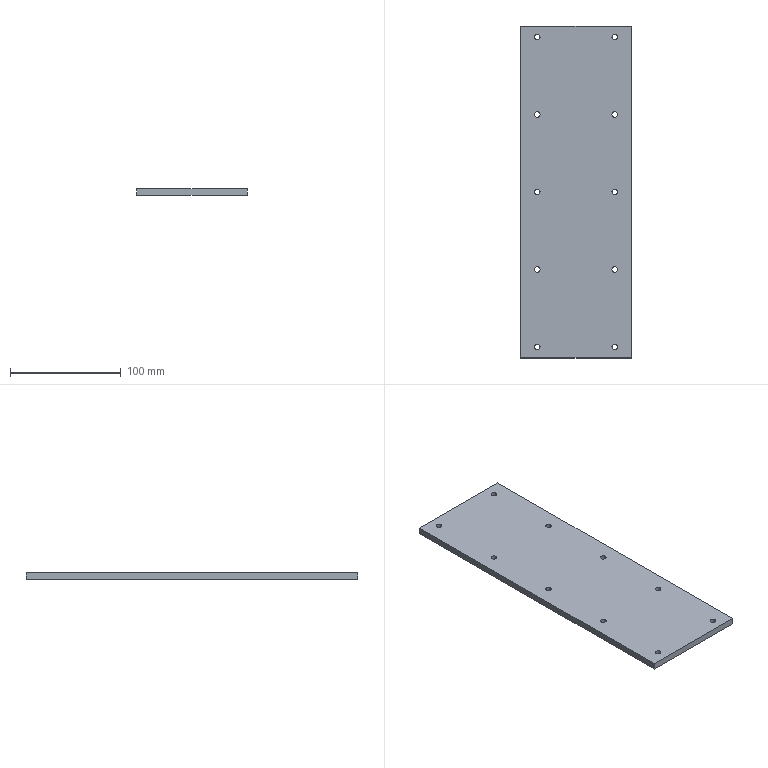Part | SolidWorks | features LPattern 2, Extrusion 1, HoleWzd 1 | 1 solid | 26 faces | box 100 x 300 x 6 mm | volume 178822 mm3 | cylinder 20 | plane 6 | commonest cylinder face diameters 5 x20
STEP:
#1=CARTESIAN_POINT('',(32.5,140.,0.));
#2=VERTEX_POINT('',#1);
#3=CARTESIAN_POINT('',(37.5,140.,0.));
#4=VERTEX_POINT('',#3);
#5=CARTESIAN_POINT('',(35.,140.,0.));
#6=DIRECTION('',(0.,0.,1.));
#7=DIRECTION('',(1.,0.,0.));
#8=AXIS2_PLACEMENT_3D('',#5,#6,#7);
#9=CIRCLE('',#8,2.5);
#10=EDGE_CURVE('',#2,#4,#9,.T.);
#11=ORIENTED_EDGE('',*,*,#10,.F.);
#12=CARTESIAN_POINT('',(32.5,140.,6.));
#13=VERTEX_POINT('',#12);
#14=CARTESIAN_POINT('',(32.5,140.,6.));
#15=DIRECTION('',(0.,0.,1.));
#16=VECTOR('',#15,1000.);
#17=LINE('',#14,#16);
#18=EDGE_CURVE('',#2,#13,#17,.T.);
#19=ORIENTED_EDGE('',*,*,#18,.T.);
#20=CARTESIAN_POINT('',(37.5,140.,6.));
#21=VERTEX_POINT('',#20);
#22=CARTESIAN_POINT('',(35.,140.,6.));
#23=DIRECTION('',(0.,0.,1.));
#24=DIRECTION('',(1.,0.,0.));
#25=AXIS2_PLACEMENT_3D('',#22,#23,#24);
#26=CIRCLE('',#25,2.5);
#27=EDGE_CURVE('',#13,#21,#26,.T.);
#28=ORIENTED_EDGE('',*,*,#27,.T.);
#29=CARTESIAN_POINT('',(37.5,140.,6.));
#30=DIRECTION('',(0.,0.,1.));
#31=VECTOR('',#30,1000.);
#32=LINE('',#29,#31);
#33=EDGE_CURVE('',#4,#21,#32,.T.);
#34=ORIENTED_EDGE('',*,*,#33,.F.);
#35=EDGE_LOOP('',(#11,#19,#28,#34));
#36=FACE_OUTER_BOUND('',#35,.T.);
#37=CARTESIAN_POINT('',(35.,140.,6.));
#38=DIRECTION('',(0.,0.,1.));
#39=DIRECTION('',(1.,0.,0.));
#40=AXIS2_PLACEMENT_3D('',#37,#38,#39);
#41=CYLINDRICAL_SURFACE('',#40,2.5);
#42=ADVANCED_FACE('',(#36),#41,.F.);
#43=CARTESIAN_POINT('',(-37.5,140.,0.));
#44=VERTEX_POINT('',#43);
#45=CARTESIAN_POINT('',(-32.5,140.,0.));
#46=VERTEX_POINT('',#45);
#47=CARTESIAN_POINT('',(-35.,140.,0.));
#48=DIRECTION('',(0.,0.,1.));
#49=DIRECTION('',(1.,0.,0.));
#50=AXIS2_PLACEMENT_3D('',#47,#48,#49);
#51=CIRCLE('',#50,2.5);
#52=EDGE_CURVE('',#44,#46,#51,.T.);
#53=ORIENTED_EDGE('',*,*,#52,.F.);
#54=CARTESIAN_POINT('',(-37.5,140.,6.));
#55=VERTEX_POINT('',#54);
#56=CARTESIAN_POINT('',(-37.5,140.,6.));
#57=DIRECTION('',(0.,0.,1.));
#58=VECTOR('',#57,1000.);
#59=LINE('',#56,#58);
#60=EDGE_CURVE('',#44,#55,#59,.T.);
#61=ORIENTED_EDGE('',*,*,#60,.T.);
#62=CARTESIAN_POINT('',(-32.5,140.,6.));
#63=VERTEX_POINT('',#62);
#64=CARTESIAN_POINT('',(-35.,140.,6.));
#65=DIRECTION('',(0.,0.,1.));
#66=DIRECTION('',(1.,0.,0.));
#67=AXIS2_PLACEMENT_3D('',#64,#65,#66);
#68=CIRCLE('',#67,2.5);
#69=EDGE_CURVE('',#55,#63,#68,.T.);
#70=ORIENTED_EDGE('',*,*,#69,.T.);
#71=CARTESIAN_POINT('',(-32.5,140.,6.));
#72=DIRECTION('',(0.,0.,1.));
#73=VECTOR('',#72,1000.);
#74=LINE('',#71,#73);
#75=EDGE_CURVE('',#46,#63,#74,.T.);
#76=ORIENTED_EDGE('',*,*,#75,.F.);
#77=EDGE_LOOP('',(#53,#61,#70,#76));
#78=FACE_OUTER_BOUND('',#77,.T.);
#79=CARTESIAN_POINT('',(-35.,140.,6.));
#80=DIRECTION('',(0.,0.,1.));
#81=DIRECTION('',(1.,0.,0.));
#82=AXIS2_PLACEMENT_3D('',#79,#80,#81);
#83=CYLINDRICAL_SURFACE('',#82,2.5);
#84=ADVANCED_FACE('',(#78),#83,.F.);
#85=CARTESIAN_POINT('',(32.5,70.,0.));
#86=VERTEX_POINT('',#85);
#87=CARTESIAN_POINT('',(37.5,70.,0.));
#88=VERTEX_POINT('',#87);
#89=CARTESIAN_POINT('',(35.,70.,0.));
#90=DIRECTION('',(0.,0.,1.));
#91=DIRECTION('',(1.,0.,0.));
#92=AXIS2_PLACEMENT_3D('',#89,#90,#91);
#93=CIRCLE('',#92,2.5);
#94=EDGE_CURVE('',#86,#88,#93,.T.);
#95=ORIENTED_EDGE('',*,*,#94,.F.);
#96=CARTESIAN_POINT('',(32.5,70.,6.));
#97=VERTEX_POINT('',#96);
#98=CARTESIAN_POINT('',(32.5,70.,6.));
#99=DIRECTION('',(0.,0.,1.));
#100=VECTOR('',#99,1000.);
#101=LINE('',#98,#100);
#102=EDGE_CURVE('',#86,#97,#101,.T.);
#103=ORIENTED_EDGE('',*,*,#102,.T.);
#104=CARTESIAN_POINT('',(37.5,70.,6.));
#105=VERTEX_POINT('',#104);
#106=CARTESIAN_POINT('',(35.,70.,6.));
#107=DIRECTION('',(0.,0.,1.));
#108=DIRECTION('',(1.,0.,0.));
#109=AXIS2_PLACEMENT_3D('',#106,#107,#108);
#110=CIRCLE('',#109,2.5);
#111=EDGE_CURVE('',#97,#105,#110,.T.);
#112=ORIENTED_EDGE('',*,*,#111,.T.);
#113=CARTESIAN_POINT('',(37.5,70.,6.));
#114=DIRECTION('',(0.,0.,1.));
#115=VECTOR('',#114,1000.);
#116=LINE('',#113,#115);
#117=EDGE_CURVE('',#88,#105,#116,.T.);
#118=ORIENTED_EDGE('',*,*,#117,.F.);
#119=EDGE_LOOP('',(#95,#103,#112,#118));
#120=FACE_OUTER_BOUND('',#119,.T.);
#121=CARTESIAN_POINT('',(35.,70.,6.));
#122=DIRECTION('',(0.,0.,1.));
#123=DIRECTION('',(1.,0.,0.));
#124=AXIS2_PLACEMENT_3D('',#121,#122,#123);
#125=CYLINDRICAL_SURFACE('',#124,2.5);
#126=ADVANCED_FACE('',(#120),#125,.F.);
#127=CARTESIAN_POINT('',(-37.5,70.,0.));
#128=VERTEX_POINT('',#127);
#129=CARTESIAN_POINT('',(-32.5,70.,0.));
#130=VERTEX_POINT('',#129);
#131=CARTESIAN_POINT('',(-35.,70.,0.));
#132=DIRECTION('',(0.,0.,1.));
#133=DIRECTION('',(1.,0.,0.));
#134=AXIS2_PLACEMENT_3D('',#131,#132,#133);
#135=CIRCLE('',#134,2.5);
#136=EDGE_CURVE('',#128,#130,#135,.T.);
#137=ORIENTED_EDGE('',*,*,#136,.F.);
#138=CARTESIAN_POINT('',(-37.5,70.,6.));
#139=VERTEX_POINT('',#138);
#140=CARTESIAN_POINT('',(-37.5,70.,6.));
#141=DIRECTION('',(0.,0.,1.));
#142=VECTOR('',#141,1000.);
#143=LINE('',#140,#142);
#144=EDGE_CURVE('',#128,#139,#143,.T.);
#145=ORIENTED_EDGE('',*,*,#144,.T.);
#146=CARTESIAN_POINT('',(-32.5,70.,6.));
#147=VERTEX_POINT('',#146);
#148=CARTESIAN_POINT('',(-35.,70.,6.));
#149=DIRECTION('',(0.,0.,1.));
#150=DIRECTION('',(1.,0.,0.));
#151=AXIS2_PLACEMENT_3D('',#148,#149,#150);
#152=CIRCLE('',#151,2.5);
#153=EDGE_CURVE('',#139,#147,#152,.T.);
#154=ORIENTED_EDGE('',*,*,#153,.T.);
#155=CARTESIAN_POINT('',(-32.5,70.,6.));
#156=DIRECTION('',(0.,0.,1.));
#157=VECTOR('',#156,1000.);
#158=LINE('',#155,#157);
#159=EDGE_CURVE('',#130,#147,#158,.T.);
#160=ORIENTED_EDGE('',*,*,#159,.F.);
#161=EDGE_LOOP('',(#137,#145,#154,#160));
#162=FACE_OUTER_BOUND('',#161,.T.);
#163=CARTESIAN_POINT('',(-35.,70.,6.));
#164=DIRECTION('',(0.,0.,1.));
#165=DIRECTION('',(1.,0.,0.));
#166=AXIS2_PLACEMENT_3D('',#163,#164,#165);
#167=CYLINDRICAL_SURFACE('',#166,2.5);
#168=ADVANCED_FACE('',(#162),#167,.F.);
#169=CARTESIAN_POINT('',(-37.5,-70.,0.));
#170=VERTEX_POINT('',#169);
#171=CARTESIAN_POINT('',(-32.5,-70.,0.));
#172=VERTEX_POINT('',#171);
#173=CARTESIAN_POINT('',(-35.,-70.,0.));
#174=DIRECTION('',(0.,0.,1.));
#175=DIRECTION('',(1.,0.,0.));
#176=AXIS2_PLACEMENT_3D('',#173,#174,#175);
#177=CIRCLE('',#176,2.5);
#178=EDGE_CURVE('',#170,#172,#177,.T.);
#179=ORIENTED_EDGE('',*,*,#178,.F.);
#180=CARTESIAN_POINT('',(-37.5,-70.,6.));
#181=VERTEX_POINT('',#180);
#182=CARTESIAN_POINT('',(-37.5,-70.,6.));
#183=DIRECTION('',(0.,0.,1.));
#184=VECTOR('',#183,1000.);
#185=LINE('',#182,#184);
#186=EDGE_CURVE('',#170,#181,#185,.T.);
#187=ORIENTED_EDGE('',*,*,#186,.T.);
#188=CARTESIAN_POINT('',(-32.5,-70.,6.));
#189=VERTEX_POINT('',#188);
#190=CARTESIAN_POINT('',(-35.,-70.,6.));
#191=DIRECTION('',(0.,0.,1.));
#192=DIRECTION('',(1.,0.,0.));
#193=AXIS2_PLACEMENT_3D('',#190,#191,#192);
#194=CIRCLE('',#193,2.5);
#195=EDGE_CURVE('',#181,#189,#194,.T.);
#196=ORIENTED_EDGE('',*,*,#195,.T.);
#197=CARTESIAN_POINT('',(-32.5,-70.,6.));
#198=DIRECTION('',(0.,0.,1.));
#199=VECTOR('',#198,1000.);
#200=LINE('',#197,#199);
#201=EDGE_CURVE('',#172,#189,#200,.T.);
#202=ORIENTED_EDGE('',*,*,#201,.F.);
#203=EDGE_LOOP('',(#179,#187,#196,#202));
#204=FACE_OUTER_BOUND('',#203,.T.);
#205=CARTESIAN_POINT('',(-35.,-70.,6.));
#206=DIRECTION('',(0.,0.,1.));
#207=DIRECTION('',(1.,0.,0.));
#208=AXIS2_PLACEMENT_3D('',#205,#206,#207);
#209=CYLINDRICAL_SURFACE('',#208,2.5);
#210=ADVANCED_FACE('',(#204),#209,.F.);
#211=CARTESIAN_POINT('',(-37.5,0.,0.));
#212=VERTEX_POINT('',#211);
#213=CARTESIAN_POINT('',(-32.5,0.,0.));
#214=VERTEX_POINT('',#213);
#215=CARTESIAN_POINT('',(-35.,0.,0.));
#216=DIRECTION('',(0.,0.,1.));
#217=DIRECTION('',(1.,0.,0.));
#218=AXIS2_PLACEMENT_3D('',#215,#216,#217);
#219=CIRCLE('',#218,2.5);
#220=EDGE_CURVE('',#212,#214,#219,.T.);
#221=ORIENTED_EDGE('',*,*,#220,.F.);
#222=CARTESIAN_POINT('',(-37.5,0.,6.));
#223=VERTEX_POINT('',#222);
#224=CARTESIAN_POINT('',(-37.5,0.,6.));
#225=DIRECTION('',(0.,0.,1.));
#226=VECTOR('',#225,1000.);
#227=LINE('',#224,#226);
#228=EDGE_CURVE('',#212,#223,#227,.T.);
#229=ORIENTED_EDGE('',*,*,#228,.T.);
#230=CARTESIAN_POINT('',(-32.5,0.,6.));
#231=VERTEX_POINT('',#230);
#232=CARTESIAN_POINT('',(-35.,0.,6.));
#233=DIRECTION('',(0.,0.,1.));
#234=DIRECTION('',(1.,0.,0.));
#235=AXIS2_PLACEMENT_3D('',#232,#233,#234);
#236=CIRCLE('',#235,2.5);
#237=EDGE_CURVE('',#223,#231,#236,.T.);
#238=ORIENTED_EDGE('',*,*,#237,.T.);
#239=CARTESIAN_POINT('',(-32.5,0.,6.));
#240=DIRECTION('',(0.,0.,1.));
#241=VECTOR('',#240,1000.);
#242=LINE('',#239,#241);
#243=EDGE_CURVE('',#214,#231,#242,.T.);
#244=ORIENTED_EDGE('',*,*,#243,.F.);
#245=EDGE_LOOP('',(#221,#229,#238,#244));
#246=FACE_OUTER_BOUND('',#245,.T.);
#247=CARTESIAN_POINT('',(-35.,0.,6.));
#248=DIRECTION('',(0.,0.,1.));
#249=DIRECTION('',(1.,0.,0.));
#250=AXIS2_PLACEMENT_3D('',#247,#248,#249);
#251=CYLINDRICAL_SURFACE('',#250,2.5);
#252=ADVANCED_FACE('',(#246),#251,.F.);
#253=CARTESIAN_POINT('',(-37.5,-140.,0.));
#254=VERTEX_POINT('',#253);
#255=CARTESIAN_POINT('',(-32.5,-140.,0.));
#256=VERTEX_POINT('',#255);
#257=CARTESIAN_POINT('',(-35.,-140.,0.));
#258=DIRECTION('',(0.,0.,1.));
#259=DIRECTION('',(1.,0.,0.));
#260=AXIS2_PLACEMENT_3D('',#257,#258,#259);
#261=CIRCLE('',#260,2.5);
#262=EDGE_CURVE('',#254,#256,#261,.T.);
#263=ORIENTED_EDGE('',*,*,#262,.F.);
#264=CARTESIAN_POINT('',(-37.5,-140.,6.));
#265=VERTEX_POINT('',#264);
#266=CARTESIAN_POINT('',(-37.5,-140.,6.));
#267=DIRECTION('',(0.,0.,1.));
#268=VECTOR('',#267,1000.);
#269=LINE('',#266,#268);
#270=EDGE_CURVE('',#254,#265,#269,.T.);
#271=ORIENTED_EDGE('',*,*,#270,.T.);
#272=CARTESIAN_POINT('',(-32.5,-140.,6.));
#273=VERTEX_POINT('',#272);
#274=CARTESIAN_POINT('',(-35.,-140.,6.));
#275=DIRECTION('',(0.,0.,1.));
#276=DIRECTION('',(1.,0.,0.));
#277=AXIS2_PLACEMENT_3D('',#274,#275,#276);
#278=CIRCLE('',#277,2.5);
#279=EDGE_CURVE('',#265,#273,#278,.T.);
#280=ORIENTED_EDGE('',*,*,#279,.T.);
#281=CARTESIAN_POINT('',(-32.5,-140.,6.));
#282=DIRECTION('',(0.,0.,1.));
#283=VECTOR('',#282,1000.);
#284=LINE('',#281,#283);
#285=EDGE_CURVE('',#256,#273,#284,.T.);
#286=ORIENTED_EDGE('',*,*,#285,.F.);
#287=EDGE_LOOP('',(#263,#271,#280,#286));
#288=FACE_OUTER_BOUND('',#287,.T.);
#289=CARTESIAN_POINT('',(-35.,-140.,6.));
#290=DIRECTION('',(0.,0.,1.));
#291=DIRECTION('',(1.,0.,0.));
#292=AXIS2_PLACEMENT_3D('',#289,#290,#291);
#293=CYLINDRICAL_SURFACE('',#292,2.5);
#294=ADVANCED_FACE('',(#288),#293,.F.);
#295=CARTESIAN_POINT('',(32.5,0.,0.));
#296=VERTEX_POINT('',#295);
#297=CARTESIAN_POINT('',(37.5,0.,0.));
#298=VERTEX_POINT('',#297);
#299=CARTESIAN_POINT('',(35.,0.,0.));
#300=DIRECTION('',(0.,0.,1.));
#301=DIRECTION('',(1.,0.,0.));
#302=AXIS2_PLACEMENT_3D('',#299,#300,#301);
#303=CIRCLE('',#302,2.5);
#304=EDGE_CURVE('',#296,#298,#303,.T.);
#305=ORIENTED_EDGE('',*,*,#304,.F.);
#306=CARTESIAN_POINT('',(32.5,0.,6.));
#307=VERTEX_POINT('',#306);
#308=CARTESIAN_POINT('',(32.5,0.,6.));
#309=DIRECTION('',(0.,0.,1.));
#310=VECTOR('',#309,1000.);
#311=LINE('',#308,#310);
#312=EDGE_CURVE('',#296,#307,#311,.T.);
#313=ORIENTED_EDGE('',*,*,#312,.T.);
#314=CARTESIAN_POINT('',(37.5,0.,6.));
#315=VERTEX_POINT('',#314);
#316=CARTESIAN_POINT('',(35.,0.,6.));
#317=DIRECTION('',(0.,0.,1.));
#318=DIRECTION('',(1.,0.,0.));
#319=AXIS2_PLACEMENT_3D('',#316,#317,#318);
#320=CIRCLE('',#319,2.5);
#321=EDGE_CURVE('',#307,#315,#320,.T.);
#322=ORIENTED_EDGE('',*,*,#321,.T.);
#323=CARTESIAN_POINT('',(37.5,0.,6.));
#324=DIRECTION('',(0.,0.,1.));
#325=VECTOR('',#324,1000.);
#326=LINE('',#323,#325);
#327=EDGE_CURVE('',#298,#315,#326,.T.);
#328=ORIENTED_EDGE('',*,*,#327,.F.);
#329=EDGE_LOOP('',(#305,#313,#322,#328));
#330=FACE_OUTER_BOUND('',#329,.T.);
#331=CARTESIAN_POINT('',(35.,0.,6.));
#332=DIRECTION('',(0.,0.,1.));
#333=DIRECTION('',(1.,0.,0.));
#334=AXIS2_PLACEMENT_3D('',#331,#332,#333);
#335=CYLINDRICAL_SURFACE('',#334,2.5);
#336=ADVANCED_FACE('',(#330),#335,.F.);
#337=CARTESIAN_POINT('',(32.5,-70.,0.));
#338=VERTEX_POINT('',#337);
#339=CARTESIAN_POINT('',(37.5,-70.,0.));
#340=VERTEX_POINT('',#339);
#341=CARTESIAN_POINT('',(35.,-70.,0.));
#342=DIRECTION('',(0.,0.,1.));
#343=DIRECTION('',(1.,0.,0.));
#344=AXIS2_PLACEMENT_3D('',#341,#342,#343);
#345=CIRCLE('',#344,2.5);
#346=EDGE_CURVE('',#338,#340,#345,.T.);
#347=ORIENTED_EDGE('',*,*,#346,.F.);
#348=CARTESIAN_POINT('',(32.5,-70.,6.));
#349=VERTEX_POINT('',#348);
#350=CARTESIAN_POINT('',(32.5,-70.,6.));
#351=DIRECTION('',(0.,0.,1.));
#352=VECTOR('',#351,1000.);
#353=LINE('',#350,#352);
#354=EDGE_CURVE('',#338,#349,#353,.T.);
#355=ORIENTED_EDGE('',*,*,#354,.T.);
#356=CARTESIAN_POINT('',(37.5,-70.,6.));
#357=VERTEX_POINT('',#356);
#358=CARTESIAN_POINT('',(35.,-70.,6.));
#359=DIRECTION('',(0.,0.,1.));
#360=DIRECTION('',(1.,0.,0.));
#361=AXIS2_PLACEMENT_3D('',#358,#359,#360);
#362=CIRCLE('',#361,2.5);
#363=EDGE_CURVE('',#349,#357,#362,.T.);
#364=ORIENTED_EDGE('',*,*,#363,.T.);
#365=CARTESIAN_POINT('',(37.5,-70.,6.));
#366=DIRECTION('',(0.,0.,1.));
#367=VECTOR('',#366,1000.);
#368=LINE('',#365,#367);
#369=EDGE_CURVE('',#340,#357,#368,.T.);
#370=ORIENTED_EDGE('',*,*,#369,.F.);
#371=EDGE_LOOP('',(#347,#355,#364,#370));
#372=FACE_OUTER_BOUND('',#371,.T.);
#373=CARTESIAN_POINT('',(35.,-70.,6.));
#374=DIRECTION('',(0.,0.,1.));
#375=DIRECTION('',(1.,0.,0.));
#376=AXIS2_PLACEMENT_3D('',#373,#374,#375);
#377=CYLINDRICAL_SURFACE('',#376,2.5);
#378=ADVANCED_FACE('',(#372),#377,.F.);
#379=CARTESIAN_POINT('',(32.5,-140.,0.));
#380=VERTEX_POINT('',#379);
#381=CARTESIAN_POINT('',(37.5,-140.,0.));
#382=VERTEX_POINT('',#381);
#383=CARTESIAN_POINT('',(35.,-140.,0.));
#384=DIRECTION('',(0.,0.,1.));
#385=DIRECTION('',(1.,0.,0.));
#386=AXIS2_PLACEMENT_3D('',#383,#384,#385);
#387=CIRCLE('',#386,2.5);
#388=EDGE_CURVE('',#380,#382,#387,.T.);
#389=ORIENTED_EDGE('',*,*,#388,.F.);
#390=CARTESIAN_POINT('',(32.5,-140.,6.));
#391=VERTEX_POINT('',#390);
#392=CARTESIAN_POINT('',(32.5,-140.,6.));
#393=DIRECTION('',(0.,0.,1.));
#394=VECTOR('',#393,1000.);
#395=LINE('',#392,#394);
#396=EDGE_CURVE('',#380,#391,#395,.T.);
#397=ORIENTED_EDGE('',*,*,#396,.T.);
#398=CARTESIAN_POINT('',(37.5,-140.,6.));
#399=VERTEX_POINT('',#398);
#400=CARTESIAN_POINT('',(35.,-140.,6.));
#401=DIRECTION('',(0.,0.,1.));
#402=DIRECTION('',(1.,0.,0.));
#403=AXIS2_PLACEMENT_3D('',#400,#401,#402);
#404=CIRCLE('',#403,2.5);
#405=EDGE_CURVE('',#391,#399,#404,.T.);
#406=ORIENTED_EDGE('',*,*,#405,.T.);
#407=CARTESIAN_POINT('',(37.5,-140.,6.));
#408=DIRECTION('',(0.,0.,1.));
#409=VECTOR('',#408,1000.);
#410=LINE('',#407,#409);
#411=EDGE_CURVE('',#382,#399,#410,.T.);
#412=ORIENTED_EDGE('',*,*,#411,.F.);
#413=EDGE_LOOP('',(#389,#397,#406,#412));
#414=FACE_OUTER_BOUND('',#413,.T.);
#415=CARTESIAN_POINT('',(35.,-140.,6.));
#416=DIRECTION('',(0.,0.,1.));
#417=DIRECTION('',(1.,0.,0.));
#418=AXIS2_PLACEMENT_3D('',#415,#416,#417);
#419=CYLINDRICAL_SURFACE('',#418,2.5);
#420=ADVANCED_FACE('',(#414),#419,.F.);
#421=CARTESIAN_POINT('',(-35.,140.,6.));
#422=DIRECTION('',(0.,0.,1.));
#423=DIRECTION('',(1.,0.,0.));
#424=AXIS2_PLACEMENT_3D('',#421,#422,#423);
#425=CIRCLE('',#424,2.5);
#426=EDGE_CURVE('',#63,#55,#425,.T.);
#427=ORIENTED_EDGE('',*,*,#426,.F.);
#428=ORIENTED_EDGE('',*,*,#69,.F.);
#429=EDGE_LOOP('',(#427,#428));
#430=FACE_BOUND('',#429,.T.);
#431=CARTESIAN_POINT('',(-35.,70.,6.));
#432=DIRECTION('',(0.,0.,1.));
#433=DIRECTION('',(1.,0.,0.));
#434=AXIS2_PLACEMENT_3D('',#431,#432,#433);
#435=CIRCLE('',#434,2.5);
#436=EDGE_CURVE('',#147,#139,#435,.T.);
#437=ORIENTED_EDGE('',*,*,#436,.F.);
#438=ORIENTED_EDGE('',*,*,#153,.F.);
#439=EDGE_LOOP('',(#437,#438));
#440=FACE_BOUND('',#439,.T.);
#441=CARTESIAN_POINT('',(-35.,-70.,6.));
#442=DIRECTION('',(0.,0.,1.));
#443=DIRECTION('',(1.,0.,0.));
#444=AXIS2_PLACEMENT_3D('',#441,#442,#443);
#445=CIRCLE('',#444,2.5);
#446=EDGE_CURVE('',#189,#181,#445,.T.);
#447=ORIENTED_EDGE('',*,*,#446,.F.);
#448=ORIENTED_EDGE('',*,*,#195,.F.);
#449=EDGE_LOOP('',(#447,#448));
#450=FACE_BOUND('',#449,.T.);
#451=CARTESIAN_POINT('',(-35.,0.,6.));
#452=DIRECTION('',(0.,0.,1.));
#453=DIRECTION('',(1.,0.,0.));
#454=AXIS2_PLACEMENT_3D('',#451,#452,#453);
#455=CIRCLE('',#454,2.5);
#456=EDGE_CURVE('',#231,#223,#455,.T.);
#457=ORIENTED_EDGE('',*,*,#456,.F.);
#458=ORIENTED_EDGE('',*,*,#237,.F.);
#459=EDGE_LOOP('',(#457,#458));
#460=FACE_BOUND('',#459,.T.);
#461=CARTESIAN_POINT('',(50.,-150.,6.));
#462=VERTEX_POINT('',#461);
#463=CARTESIAN_POINT('',(50.,150.,6.));
#464=VERTEX_POINT('',#463);
#465=CARTESIAN_POINT('',(50.,-150.,6.));
#466=DIRECTION('',(0.,1.,0.));
#467=VECTOR('',#466,1000.);
#468=LINE('',#465,#467);
#469=EDGE_CURVE('',#462,#464,#468,.T.);
#470=ORIENTED_EDGE('',*,*,#469,.T.);
#471=CARTESIAN_POINT('',(-50.,150.,6.));
#472=VERTEX_POINT('',#471);
#473=CARTESIAN_POINT('',(-50.,150.,6.));
#474=DIRECTION('',(-1.,0.,0.));
#475=VECTOR('',#474,1000.);
#476=LINE('',#473,#475);
#477=EDGE_CURVE('',#464,#472,#476,.T.);
#478=ORIENTED_EDGE('',*,*,#477,.T.);
#479=CARTESIAN_POINT('',(-50.,-150.,6.));
#480=VERTEX_POINT('',#479);
#481=CARTESIAN_POINT('',(-50.,-150.,6.));
#482=DIRECTION('',(0.,-1.,0.));
#483=VECTOR('',#482,1000.);
#484=LINE('',#481,#483);
#485=EDGE_CURVE('',#472,#480,#484,.T.);
#486=ORIENTED_EDGE('',*,*,#485,.T.);
#487=CARTESIAN_POINT('',(-50.,-150.,6.));
#488=DIRECTION('',(1.,0.,0.));
#489=VECTOR('',#488,1000.);
#490=LINE('',#487,#489);
#491=EDGE_CURVE('',#480,#462,#490,.T.);
#492=ORIENTED_EDGE('',*,*,#491,.T.);
#493=EDGE_LOOP('',(#470,#478,#486,#492));
#494=FACE_OUTER_BOUND('',#493,.T.);
#495=CARTESIAN_POINT('',(-35.,-140.,6.));
#496=DIRECTION('',(0.,0.,1.));
#497=DIRECTION('',(1.,0.,0.));
#498=AXIS2_PLACEMENT_3D('',#495,#496,#497);
#499=CIRCLE('',#498,2.5);
#500=EDGE_CURVE('',#273,#265,#499,.T.);
#501=ORIENTED_EDGE('',*,*,#500,.F.);
#502=ORIENTED_EDGE('',*,*,#279,.F.);
#503=EDGE_LOOP('',(#501,#502));
#504=FACE_BOUND('',#503,.T.);
#505=CARTESIAN_POINT('',(35.,0.,6.));
#506=DIRECTION('',(0.,0.,1.));
#507=DIRECTION('',(1.,0.,0.));
#508=AXIS2_PLACEMENT_3D('',#505,#506,#507);
#509=CIRCLE('',#508,2.5);
#510=EDGE_CURVE('',#315,#307,#509,.T.);
#511=ORIENTED_EDGE('',*,*,#510,.F.);
#512=ORIENTED_EDGE('',*,*,#321,.F.);
#513=EDGE_LOOP('',(#511,#512));
#514=FACE_BOUND('',#513,.T.);
#515=CARTESIAN_POINT('',(35.,-70.,6.));
#516=DIRECTION('',(0.,0.,1.));
#517=DIRECTION('',(1.,0.,0.));
#518=AXIS2_PLACEMENT_3D('',#515,#516,#517);
#519=CIRCLE('',#518,2.5);
#520=EDGE_CURVE('',#357,#349,#519,.T.);
#521=ORIENTED_EDGE('',*,*,#520,.F.);
#522=ORIENTED_EDGE('',*,*,#363,.F.);
#523=EDGE_LOOP('',(#521,#522));
#524=FACE_BOUND('',#523,.T.);
#525=CARTESIAN_POINT('',(35.,-140.,6.));
#526=DIRECTION('',(0.,0.,1.));
#527=DIRECTION('',(1.,0.,0.));
#528=AXIS2_PLACEMENT_3D('',#525,#526,#527);
#529=CIRCLE('',#528,2.5);
#530=EDGE_CURVE('',#399,#391,#529,.T.);
#531=ORIENTED_EDGE('',*,*,#530,.F.);
#532=ORIENTED_EDGE('',*,*,#405,.F.);
#533=EDGE_LOOP('',(#531,#532));
#534=FACE_BOUND('',#533,.T.);
#535=CARTESIAN_POINT('',(35.,70.,6.));
#536=DIRECTION('',(0.,0.,1.));
#537=DIRECTION('',(1.,0.,0.));
#538=AXIS2_PLACEMENT_3D('',#535,#536,#537);
#539=CIRCLE('',#538,2.5);
#540=EDGE_CURVE('',#105,#97,#539,.T.);
#541=ORIENTED_EDGE('',*,*,#540,.F.);
#542=ORIENTED_EDGE('',*,*,#111,.F.);
#543=EDGE_LOOP('',(#541,#542));
#544=FACE_BOUND('',#543,.T.);
#545=CARTESIAN_POINT('',(35.,140.,6.));
#546=DIRECTION('',(0.,0.,1.));
#547=DIRECTION('',(1.,0.,0.));
#548=AXIS2_PLACEMENT_3D('',#545,#546,#547);
#549=CIRCLE('',#548,2.5);
#550=EDGE_CURVE('',#21,#13,#549,.T.);
#551=ORIENTED_EDGE('',*,*,#550,.F.);
#552=ORIENTED_EDGE('',*,*,#27,.F.);
#553=EDGE_LOOP('',(#551,#552));
#554=FACE_BOUND('',#553,.T.);
#555=CARTESIAN_POINT('',(0.,0.,6.));
#556=DIRECTION('',(0.,0.,-1.));
#557=DIRECTION('',(-1.,0.,0.));
#558=AXIS2_PLACEMENT_3D('',#555,#556,#557);
#559=PLANE('',#558);
#560=ADVANCED_FACE('',(#430,#440,#450,#460,#494,#504,#514,#524,#534,#544,#554),#559,.F.);
#561=CARTESIAN_POINT('',(35.,140.,0.));
#562=DIRECTION('',(0.,0.,1.));
#563=DIRECTION('',(1.,0.,0.));
#564=AXIS2_PLACEMENT_3D('',#561,#562,#563);
#565=CIRCLE('',#564,2.5);
#566=EDGE_CURVE('',#4,#2,#565,.T.);
#567=ORIENTED_EDGE('',*,*,#566,.T.);
#568=ORIENTED_EDGE('',*,*,#10,.T.);
#569=EDGE_LOOP('',(#567,#568));
#570=FACE_BOUND('',#569,.T.);
#571=CARTESIAN_POINT('',(35.,70.,0.));
#572=DIRECTION('',(0.,0.,1.));
#573=DIRECTION('',(1.,0.,0.));
#574=AXIS2_PLACEMENT_3D('',#571,#572,#573);
#575=CIRCLE('',#574,2.5);
#576=EDGE_CURVE('',#88,#86,#575,.T.);
#577=ORIENTED_EDGE('',*,*,#576,.T.);
#578=ORIENTED_EDGE('',*,*,#94,.T.);
#579=EDGE_LOOP('',(#577,#578));
#580=FACE_BOUND('',#579,.T.);
#581=CARTESIAN_POINT('',(-35.,70.,0.));
#582=DIRECTION('',(0.,0.,1.));
#583=DIRECTION('',(1.,0.,0.));
#584=AXIS2_PLACEMENT_3D('',#581,#582,#583);
#585=CIRCLE('',#584,2.5);
#586=EDGE_CURVE('',#130,#128,#585,.T.);
#587=ORIENTED_EDGE('',*,*,#586,.T.);
#588=ORIENTED_EDGE('',*,*,#136,.T.);
#589=EDGE_LOOP('',(#587,#588));
#590=FACE_BOUND('',#589,.T.);
#591=CARTESIAN_POINT('',(-35.,-70.,0.));
#592=DIRECTION('',(0.,0.,1.));
#593=DIRECTION('',(1.,0.,0.));
#594=AXIS2_PLACEMENT_3D('',#591,#592,#593);
#595=CIRCLE('',#594,2.5);
#596=EDGE_CURVE('',#172,#170,#595,.T.);
#597=ORIENTED_EDGE('',*,*,#596,.T.);
#598=ORIENTED_EDGE('',*,*,#178,.T.);
#599=EDGE_LOOP('',(#597,#598));
#600=FACE_BOUND('',#599,.T.);
#601=CARTESIAN_POINT('',(-35.,0.,0.));
#602=DIRECTION('',(0.,0.,1.));
#603=DIRECTION('',(1.,0.,0.));
#604=AXIS2_PLACEMENT_3D('',#601,#602,#603);
#605=CIRCLE('',#604,2.5);
#606=EDGE_CURVE('',#214,#212,#605,.T.);
#607=ORIENTED_EDGE('',*,*,#606,.T.);
#608=ORIENTED_EDGE('',*,*,#220,.T.);
#609=EDGE_LOOP('',(#607,#608));
#610=FACE_BOUND('',#609,.T.);
#611=CARTESIAN_POINT('',(50.,-150.,0.));
#612=VERTEX_POINT('',#611);
#613=CARTESIAN_POINT('',(50.,150.,0.));
#614=VERTEX_POINT('',#613);
#615=CARTESIAN_POINT('',(50.,-150.,0.));
#616=DIRECTION('',(0.,1.,0.));
#617=VECTOR('',#616,1000.);
#618=LINE('',#615,#617);
#619=EDGE_CURVE('',#612,#614,#618,.T.);
#620=ORIENTED_EDGE('',*,*,#619,.F.);
#621=CARTESIAN_POINT('',(-50.,-150.,0.));
#622=VERTEX_POINT('',#621);
#623=CARTESIAN_POINT('',(-50.,-150.,0.));
#624=DIRECTION('',(1.,0.,0.));
#625=VECTOR('',#624,1000.);
#626=LINE('',#623,#625);
#627=EDGE_CURVE('',#622,#612,#626,.T.);
#628=ORIENTED_EDGE('',*,*,#627,.F.);
#629=CARTESIAN_POINT('',(-50.,150.,0.));
#630=VERTEX_POINT('',#629);
#631=CARTESIAN_POINT('',(-50.,-150.,0.));
#632=DIRECTION('',(0.,-1.,0.));
#633=VECTOR('',#632,1000.);
#634=LINE('',#631,#633);
#635=EDGE_CURVE('',#630,#622,#634,.T.);
#636=ORIENTED_EDGE('',*,*,#635,.F.);
#637=CARTESIAN_POINT('',(-50.,150.,0.));
#638=DIRECTION('',(-1.,0.,0.));
#639=VECTOR('',#638,1000.);
#640=LINE('',#637,#639);
#641=EDGE_CURVE('',#614,#630,#640,.T.);
#642=ORIENTED_EDGE('',*,*,#641,.F.);
#643=EDGE_LOOP('',(#620,#628,#636,#642));
#644=FACE_OUTER_BOUND('',#643,.T.);
#645=CARTESIAN_POINT('',(-35.,-140.,0.));
#646=DIRECTION('',(0.,0.,1.));
#647=DIRECTION('',(1.,0.,0.));
#648=AXIS2_PLACEMENT_3D('',#645,#646,#647);
#649=CIRCLE('',#648,2.5);
#650=EDGE_CURVE('',#256,#254,#649,.T.);
#651=ORIENTED_EDGE('',*,*,#650,.T.);
#652=ORIENTED_EDGE('',*,*,#262,.T.);
#653=EDGE_LOOP('',(#651,#652));
#654=FACE_BOUND('',#653,.T.);
#655=CARTESIAN_POINT('',(35.,0.,0.));
#656=DIRECTION('',(0.,0.,1.));
#657=DIRECTION('',(1.,0.,0.));
#658=AXIS2_PLACEMENT_3D('',#655,#656,#657);
#659=CIRCLE('',#658,2.5);
#660=EDGE_CURVE('',#298,#296,#659,.T.);
#661=ORIENTED_EDGE('',*,*,#660,.T.);
#662=ORIENTED_EDGE('',*,*,#304,.T.);
#663=EDGE_LOOP('',(#661,#662));
#664=FACE_BOUND('',#663,.T.);
#665=CARTESIAN_POINT('',(35.,-70.,0.));
#666=DIRECTION('',(0.,0.,1.));
#667=DIRECTION('',(1.,0.,0.));
#668=AXIS2_PLACEMENT_3D('',#665,#666,#667);
#669=CIRCLE('',#668,2.5);
#670=EDGE_CURVE('',#340,#338,#669,.T.);
#671=ORIENTED_EDGE('',*,*,#670,.T.);
#672=ORIENTED_EDGE('',*,*,#346,.T.);
#673=EDGE_LOOP('',(#671,#672));
#674=FACE_BOUND('',#673,.T.);
#675=CARTESIAN_POINT('',(35.,-140.,0.));
#676=DIRECTION('',(0.,0.,1.));
#677=DIRECTION('',(1.,0.,0.));
#678=AXIS2_PLACEMENT_3D('',#675,#676,#677);
#679=CIRCLE('',#678,2.5);
#680=EDGE_CURVE('',#382,#380,#679,.T.);
#681=ORIENTED_EDGE('',*,*,#680,.T.);
#682=ORIENTED_EDGE('',*,*,#388,.T.);
#683=EDGE_LOOP('',(#681,#682));
#684=FACE_BOUND('',#683,.T.);
#685=CARTESIAN_POINT('',(-35.,140.,0.));
#686=DIRECTION('',(0.,0.,1.));
#687=DIRECTION('',(1.,0.,0.));
#688=AXIS2_PLACEMENT_3D('',#685,#686,#687);
#689=CIRCLE('',#688,2.5);
#690=EDGE_CURVE('',#46,#44,#689,.T.);
#691=ORIENTED_EDGE('',*,*,#690,.T.);
#692=ORIENTED_EDGE('',*,*,#52,.T.);
#693=EDGE_LOOP('',(#691,#692));
#694=FACE_BOUND('',#693,.T.);
#695=CARTESIAN_POINT('',(0.,0.,0.));
#696=DIRECTION('',(0.,0.,-1.));
#697=DIRECTION('',(-1.,0.,0.));
#698=AXIS2_PLACEMENT_3D('',#695,#696,#697);
#699=PLANE('',#698);
#700=ADVANCED_FACE('',(#570,#580,#590,#600,#610,#644,#654,#664,#674,#684,#694),#699,.T.);
#701=ORIENTED_EDGE('',*,*,#396,.F.);
#702=ORIENTED_EDGE('',*,*,#680,.F.);
#703=ORIENTED_EDGE('',*,*,#411,.T.);
#704=ORIENTED_EDGE('',*,*,#530,.T.);
#705=EDGE_LOOP('',(#701,#702,#703,#704));
#706=FACE_OUTER_BOUND('',#705,.T.);
#707=CARTESIAN_POINT('',(35.,-140.,6.));
#708=DIRECTION('',(0.,0.,1.));
#709=DIRECTION('',(1.,0.,0.));
#710=AXIS2_PLACEMENT_3D('',#707,#708,#709);
#711=CYLINDRICAL_SURFACE('',#710,2.5);
#712=ADVANCED_FACE('',(#706),#711,.F.);
#713=ORIENTED_EDGE('',*,*,#354,.F.);
#714=ORIENTED_EDGE('',*,*,#670,.F.);
#715=ORIENTED_EDGE('',*,*,#369,.T.);
#716=ORIENTED_EDGE('',*,*,#520,.T.);
#717=EDGE_LOOP('',(#713,#714,#715,#716));
#718=FACE_OUTER_BOUND('',#717,.T.);
#719=CARTESIAN_POINT('',(35.,-70.,6.));
#720=DIRECTION('',(0.,0.,1.));
#721=DIRECTION('',(1.,0.,0.));
#722=AXIS2_PLACEMENT_3D('',#719,#720,#721);
#723=CYLINDRICAL_SURFACE('',#722,2.5);
#724=ADVANCED_FACE('',(#718),#723,.F.);
#725=ORIENTED_EDGE('',*,*,#312,.F.);
#726=ORIENTED_EDGE('',*,*,#660,.F.);
#727=ORIENTED_EDGE('',*,*,#327,.T.);
#728=ORIENTED_EDGE('',*,*,#510,.T.);
#729=EDGE_LOOP('',(#725,#726,#727,#728));
#730=FACE_OUTER_BOUND('',#729,.T.);
#731=CARTESIAN_POINT('',(35.,0.,6.));
#732=DIRECTION('',(0.,0.,1.));
#733=DIRECTION('',(1.,0.,0.));
#734=AXIS2_PLACEMENT_3D('',#731,#732,#733);
#735=CYLINDRICAL_SURFACE('',#734,2.5);
#736=ADVANCED_FACE('',(#730),#735,.F.);
#737=ORIENTED_EDGE('',*,*,#270,.F.);
#738=ORIENTED_EDGE('',*,*,#650,.F.);
#739=ORIENTED_EDGE('',*,*,#285,.T.);
#740=ORIENTED_EDGE('',*,*,#500,.T.);
#741=EDGE_LOOP('',(#737,#738,#739,#740));
#742=FACE_OUTER_BOUND('',#741,.T.);
#743=CARTESIAN_POINT('',(-35.,-140.,6.));
#744=DIRECTION('',(0.,0.,1.));
#745=DIRECTION('',(1.,0.,0.));
#746=AXIS2_PLACEMENT_3D('',#743,#744,#745);
#747=CYLINDRICAL_SURFACE('',#746,2.5);
#748=ADVANCED_FACE('',(#742),#747,.F.);
#749=ORIENTED_EDGE('',*,*,#619,.T.);
#750=CARTESIAN_POINT('',(50.,150.,6.));
#751=DIRECTION('',(0.,0.,-1.));
#752=VECTOR('',#751,1000.);
#753=LINE('',#750,#752);
#754=EDGE_CURVE('',#464,#614,#753,.T.);
#755=ORIENTED_EDGE('',*,*,#754,.F.);
#756=ORIENTED_EDGE('',*,*,#469,.F.);
#757=CARTESIAN_POINT('',(50.,-150.,6.));
#758=DIRECTION('',(0.,0.,-1.));
#759=VECTOR('',#758,1000.);
#760=LINE('',#757,#759);
#761=EDGE_CURVE('',#462,#612,#760,.T.);
#762=ORIENTED_EDGE('',*,*,#761,.T.);
#763=EDGE_LOOP('',(#749,#755,#756,#762));
#764=FACE_OUTER_BOUND('',#763,.T.);
#765=CARTESIAN_POINT('',(50.,-150.,6.));
#766=DIRECTION('',(-1.,0.,0.));
#767=DIRECTION('',(0.,0.,1.));
#768=AXIS2_PLACEMENT_3D('',#765,#766,#767);
#769=PLANE('',#768);
#770=ADVANCED_FACE('',(#764),#769,.F.);
#771=ORIENTED_EDGE('',*,*,#641,.T.);
#772=CARTESIAN_POINT('',(-50.,150.,6.));
#773=DIRECTION('',(0.,0.,-1.));
#774=VECTOR('',#773,1000.);
#775=LINE('',#772,#774);
#776=EDGE_CURVE('',#472,#630,#775,.T.);
#777=ORIENTED_EDGE('',*,*,#776,.F.);
#778=ORIENTED_EDGE('',*,*,#477,.F.);
#779=ORIENTED_EDGE('',*,*,#754,.T.);
#780=EDGE_LOOP('',(#771,#777,#778,#779));
#781=FACE_OUTER_BOUND('',#780,.T.);
#782=CARTESIAN_POINT('',(-50.,150.,6.));
#783=DIRECTION('',(0.,-1.,0.));
#784=DIRECTION('',(0.,0.,-1.));
#785=AXIS2_PLACEMENT_3D('',#782,#783,#784);
#786=PLANE('',#785);
#787=ADVANCED_FACE('',(#781),#786,.F.);
#788=ORIENTED_EDGE('',*,*,#635,.T.);
#789=CARTESIAN_POINT('',(-50.,-150.,6.));
#790=DIRECTION('',(0.,0.,-1.));
#791=VECTOR('',#790,1000.);
#792=LINE('',#789,#791);
#793=EDGE_CURVE('',#480,#622,#792,.T.);
#794=ORIENTED_EDGE('',*,*,#793,.F.);
#795=ORIENTED_EDGE('',*,*,#485,.F.);
#796=ORIENTED_EDGE('',*,*,#776,.T.);
#797=EDGE_LOOP('',(#788,#794,#795,#796));
#798=FACE_OUTER_BOUND('',#797,.T.);
#799=CARTESIAN_POINT('',(-50.,-150.,6.));
#800=DIRECTION('',(1.,0.,0.));
#801=DIRECTION('',(0.,0.,-1.));
#802=AXIS2_PLACEMENT_3D('',#799,#800,#801);
#803=PLANE('',#802);
#804=ADVANCED_FACE('',(#798),#803,.F.);
#805=ORIENTED_EDGE('',*,*,#627,.T.);
#806=ORIENTED_EDGE('',*,*,#761,.F.);
#807=ORIENTED_EDGE('',*,*,#491,.F.);
#808=ORIENTED_EDGE('',*,*,#793,.T.);
#809=EDGE_LOOP('',(#805,#806,#807,#808));
#810=FACE_OUTER_BOUND('',#809,.T.);
#811=CARTESIAN_POINT('',(-50.,-150.,6.));
#812=DIRECTION('',(0.,1.,0.));
#813=DIRECTION('',(0.,0.,1.));
#814=AXIS2_PLACEMENT_3D('',#811,#812,#813);
#815=PLANE('',#814);
#816=ADVANCED_FACE('',(#810),#815,.F.);
#817=ORIENTED_EDGE('',*,*,#228,.F.);
#818=ORIENTED_EDGE('',*,*,#606,.F.);
#819=ORIENTED_EDGE('',*,*,#243,.T.);
#820=ORIENTED_EDGE('',*,*,#456,.T.);
#821=EDGE_LOOP('',(#817,#818,#819,#820));
#822=FACE_OUTER_BOUND('',#821,.T.);
#823=CARTESIAN_POINT('',(-35.,0.,6.));
#824=DIRECTION('',(0.,0.,1.));
#825=DIRECTION('',(1.,0.,0.));
#826=AXIS2_PLACEMENT_3D('',#823,#824,#825);
#827=CYLINDRICAL_SURFACE('',#826,2.5);
#828=ADVANCED_FACE('',(#822),#827,.F.);
#829=ORIENTED_EDGE('',*,*,#186,.F.);
#830=ORIENTED_EDGE('',*,*,#596,.F.);
#831=ORIENTED_EDGE('',*,*,#201,.T.);
#832=ORIENTED_EDGE('',*,*,#446,.T.);
#833=EDGE_LOOP('',(#829,#830,#831,#832));
#834=FACE_OUTER_BOUND('',#833,.T.);
#835=CARTESIAN_POINT('',(-35.,-70.,6.));
#836=DIRECTION('',(0.,0.,1.));
#837=DIRECTION('',(1.,0.,0.));
#838=AXIS2_PLACEMENT_3D('',#835,#836,#837);
#839=CYLINDRICAL_SURFACE('',#838,2.5);
#840=ADVANCED_FACE('',(#834),#839,.F.);
#841=ORIENTED_EDGE('',*,*,#144,.F.);
#842=ORIENTED_EDGE('',*,*,#586,.F.);
#843=ORIENTED_EDGE('',*,*,#159,.T.);
#844=ORIENTED_EDGE('',*,*,#436,.T.);
#845=EDGE_LOOP('',(#841,#842,#843,#844));
#846=FACE_OUTER_BOUND('',#845,.T.);
#847=CARTESIAN_POINT('',(-35.,70.,6.));
#848=DIRECTION('',(0.,0.,1.));
#849=DIRECTION('',(1.,0.,0.));
#850=AXIS2_PLACEMENT_3D('',#847,#848,#849);
#851=CYLINDRICAL_SURFACE('',#850,2.5);
#852=ADVANCED_FACE('',(#846),#851,.F.);
#853=ORIENTED_EDGE('',*,*,#102,.F.);
#854=ORIENTED_EDGE('',*,*,#576,.F.);
#855=ORIENTED_EDGE('',*,*,#117,.T.);
#856=ORIENTED_EDGE('',*,*,#540,.T.);
#857=EDGE_LOOP('',(#853,#854,#855,#856));
#858=FACE_OUTER_BOUND('',#857,.T.);
#859=CARTESIAN_POINT('',(35.,70.,6.));
#860=DIRECTION('',(0.,0.,1.));
#861=DIRECTION('',(1.,0.,0.));
#862=AXIS2_PLACEMENT_3D('',#859,#860,#861);
#863=CYLINDRICAL_SURFACE('',#862,2.5);
#864=ADVANCED_FACE('',(#858),#863,.F.);
#865=ORIENTED_EDGE('',*,*,#60,.F.);
#866=ORIENTED_EDGE('',*,*,#690,.F.);
#867=ORIENTED_EDGE('',*,*,#75,.T.);
#868=ORIENTED_EDGE('',*,*,#426,.T.);
#869=EDGE_LOOP('',(#865,#866,#867,#868));
#870=FACE_OUTER_BOUND('',#869,.T.);
#871=CARTESIAN_POINT('',(-35.,140.,6.));
#872=DIRECTION('',(0.,0.,1.));
#873=DIRECTION('',(1.,0.,0.));
#874=AXIS2_PLACEMENT_3D('',#871,#872,#873);
#875=CYLINDRICAL_SURFACE('',#874,2.5);
#876=ADVANCED_FACE('',(#870),#875,.F.);
#877=ORIENTED_EDGE('',*,*,#18,.F.);
#878=ORIENTED_EDGE('',*,*,#566,.F.);
#879=ORIENTED_EDGE('',*,*,#33,.T.);
#880=ORIENTED_EDGE('',*,*,#550,.T.);
#881=EDGE_LOOP('',(#877,#878,#879,#880));
#882=FACE_OUTER_BOUND('',#881,.T.);
#883=CARTESIAN_POINT('',(35.,140.,6.));
#884=DIRECTION('',(0.,0.,1.));
#885=DIRECTION('',(1.,0.,0.));
#886=AXIS2_PLACEMENT_3D('',#883,#884,#885);
#887=CYLINDRICAL_SURFACE('',#886,2.5);
#888=ADVANCED_FACE('',(#882),#887,.F.);
#889=CLOSED_SHELL('',(#42,#84,#126,#168,#210,#252,#294,#336,#378,#420,#560,#700,#712,#724,#736,#748,#770,#787,#804,#816,#828,#840,#852,#864,#876,#888));
#890=MANIFOLD_SOLID_BREP('',#889);
#891=CARTESIAN_POINT('',(0.,0.,0.));
#892=DIRECTION('',(0.,0.,1.));
#893=DIRECTION('',(1.,0.,0.));
#894=AXIS2_PLACEMENT_3D('',#891,#892,#893);
#895=(LENGTH_UNIT()NAMED_UNIT(*)SI_UNIT(.MILLI.,.METRE.));
#896=UNCERTAINTY_MEASURE_WITH_UNIT(LENGTH_MEASURE(0.00001),#895,'','');
#897=(NAMED_UNIT(*)PLANE_ANGLE_UNIT()SI_UNIT($,.RADIAN.));
#898=(NAMED_UNIT(*)SI_UNIT($,.STERADIAN.)SOLID_ANGLE_UNIT());
#899=(GEOMETRIC_REPRESENTATION_CONTEXT(3)GLOBAL_UNCERTAINTY_ASSIGNED_CONTEXT((#896))GLOBAL_UNIT_ASSIGNED_CONTEXT((#895,#897,#898))REPRESENTATION_CONTEXT('',''));
#900=ADVANCED_BREP_SHAPE_REPRESENTATION('',(#890,#894),#899);